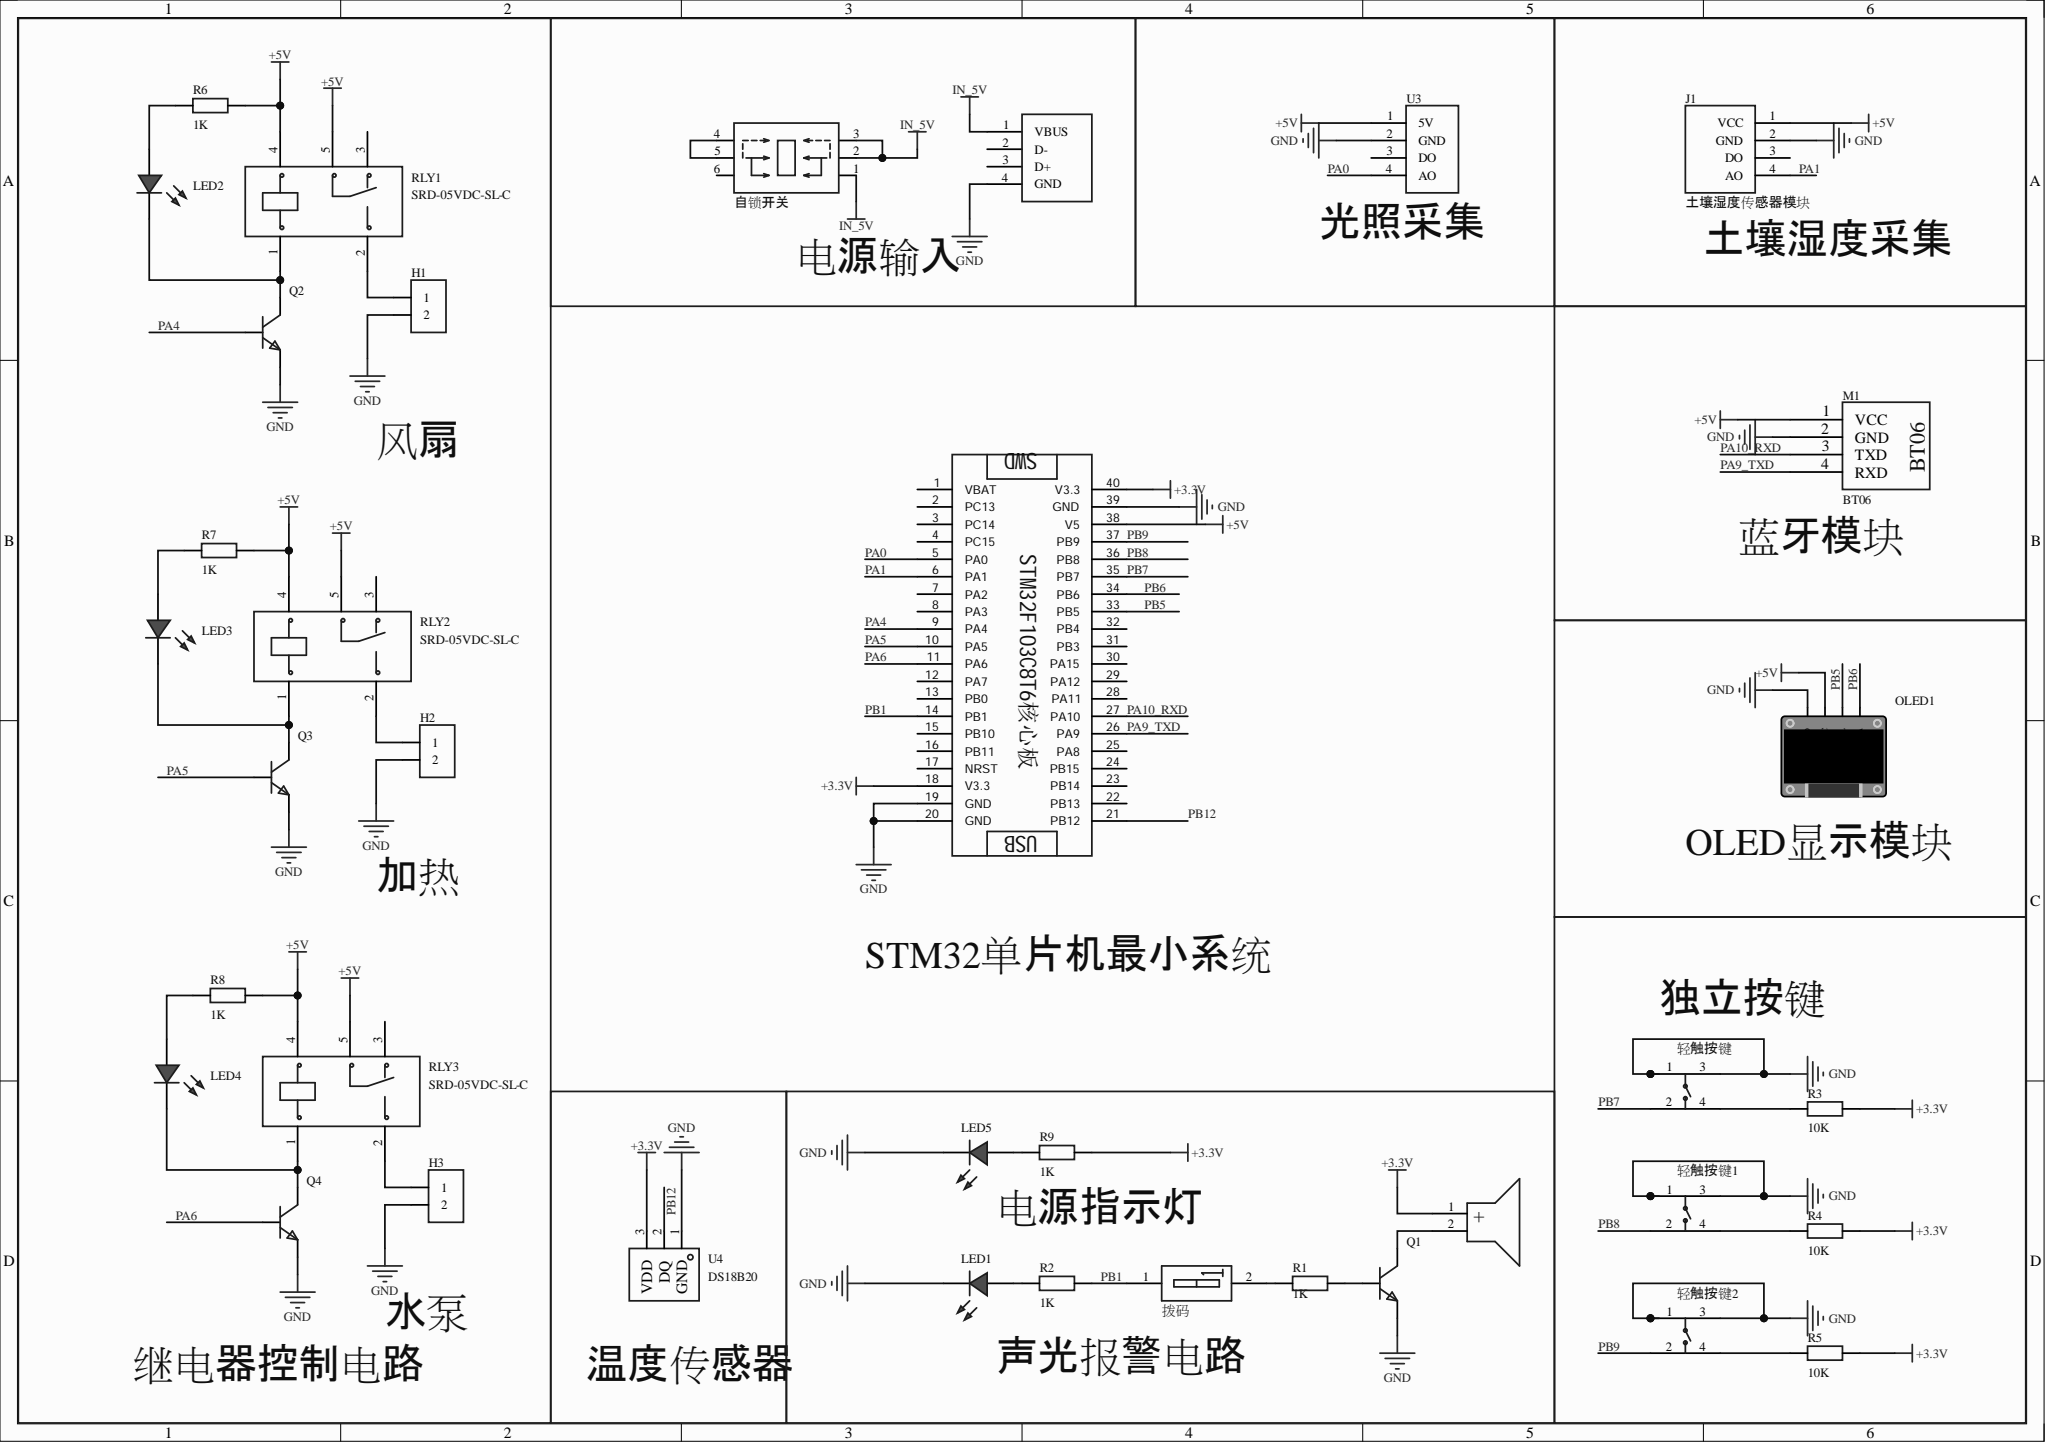Circuit board | Altium Designer | 37 parts | 36 nets
Bill of materials:
Comment,Description,Designator,Footprint,LibRef,Quantity
"3kHz","驱动方式:有源(内含驱动线路);构造类型:电磁式;频率:3kHz;声压(SPL):85dB;","BUZZER1","BUZ-TH_BD9.0-P5.00-D0.6-FD","HNB09A03","1"
"","","H1, H2, H3","HDR-TH_2P-P2.54-V-F","HDR-F_2.54_1x2P","3"
"土壤湿度传感器模块","","J1","Hearder-4","土壤湿度传感器模块","1"
"","","LED1, LED2, LED3, LED4, LED5","LED-TH_5mm","LED_TH-R_5mm","5"
"BT06","","M1","BT06","BT06","1"
"","","OLED1","0.96OLED_4P","0.96OLED模块_4P","1"
"S8050","晶体管类型:NPN;集电极电流(Ic):500mA;集射极击穿电压(Vceo):25V;耗散功率(Pd):300mW;直流电流增益(hFE):120@50mA,1.0V;","Q1, Q2, Q3, Q4","SOT-23-3_L2.9-W1.3-P1.90-LS2.3-BR","S8050_C20069125","4"
"1K","","R1, R2, R6, R7, R8, R9","R0805","Res_0805","6"
"10K","","R3, R4, R5","R0805","Res_0805","3"
"SRD-05VDC-SL-C","线圈电压:5V;触点形式:一组转换:1C(单刀双掷-转换);触点容量(电阻负载):-;最大切换电压:250V@AC;最大切换电流:15A;","RLY1, RLY2, RLY3","RELAY-TH_SRD-XXVDC-XL-C","SRD-05VDC-SL-C","3"
"自锁开关","8.5x8.5x14，6只端子、自锁、底座黑色、盖板灰色","SW1","SW-TH_6P-L8.5-W8.5-P2.50-LS5.5-BL-2","PS851-06L140E1-ZCY-G","1"
"拨码","类型:平拨,凸起式;电路结构:单刀单掷;开关位数:1位;工作寿命:-;颜色:红色;","SW2","SW-TH_DSWB01LHGET","DSWB01LHGET","1"
"","","U1","USB-type-C模块","TYPE-C模块","1"
"CW32F030C8最小系统板","","U2","STM32F103C8T6核心板","STM32F103C8T6最小系统","1"
"","","U3","光敏传感器模块","光敏传感器模块","1"
"DS18B20","","U4","3p_2.54","DS18B20","1"
"SH-6X6X6.5H-TP","电路结构:单刀单掷;按钮形状:圆形按钮;作用力:2.5N;安装方式:立贴;开关长度:6mm;开关宽度:6mm;开关高度:6.5mm;带支架:不带支架;触点电流:50mA;额定电压:12V;带灯:无;工作寿命:10万次;","轻触按键","SW-SMD_4P-L6.2-W6.2-P4.50-LS9.5-TL","SH-6X6X6.5H-TP","1"
"SH-6X6X6.5H-TP","电路结构:单刀单掷;按钮形状:圆形按钮;作用力:2.5N;安装方式:立贴;开关长度:6mm;开关宽度:6mm;开关高度:6.5mm;带支架:不带支架;触点电流:50mA;额定电压:12V;带灯:无;工作寿命:10万次;","轻触按键1, 轻触按键2","SW-SMD_4P-L6.0-W6.0-P4.50-LS8.8","SH-6X6X6.5H-TP","2"
Netlist (Protel format):
[
BUZZER1
BUZ-TH_BD9.0-P5.00-D0.6-FD
3kHz



]
[
H1
HDR-TH_2P-P2.54-V-F




]
[
H2
HDR-TH_2P-P2.54-V-F




]
[
H3
HDR-TH_2P-P2.54-V-F




]
[
J1
Hearder-4
土壤湿度传感器模块



]
[
LED1
LED-TH_5mm




]
[
LED2
LED-TH_5mm




]
[
LED3
LED-TH_5mm




]
[
LED4
LED-TH_5mm




]
[
LED5
LED-TH_5mm




]
[
M1
BT06
BT06



]
[
OLED1
0.96OLED_4P




]
[
Q1
SOT-23-3_L2.9-W1.3-P1.90-LS2.3-BR
S8050



]
[
Q2
SOT-23-3_L2.9-W1.3-P1.90-LS2.3-BR
S8050



]
[
Q3
SOT-23-3_L2.9-W1.3-P1.90-LS2.3-BR
S8050



]
[
Q4
SOT-23-3_L2.9-W1.3-P1.90-LS2.3-BR
S8050



]
[
R1
R0805
1K



]
[
R2
R0805
1K



]
[
R3
R0805
10K



]
[
R4
R0805
10K



]
[
R5
R0805
10K



]
[
R6
R0805
1K



]
[
R7
R0805
1K



]
[
R8
R0805
1K



]
[
R9
R0805
1K



]
[
RLY1
RELAY-TH_SRD-XXVDC-XL-C
SRD-05VDC-SL-C



]
[
RLY2
RELAY-TH_SRD-XXVDC-XL-C
SRD-05VDC-SL-C



]
[
RLY3
RELAY-TH_SRD-XXVDC-XL-C
SRD-05VDC-SL-C



]
[
SW1
SW-TH_6P-L8.5-W8.5-P2.50-LS5.5-BL-2
自锁开关



]
[
SW2
SW-TH_DSWB01LHGET
拨码



]
[
U1
USB-type-C模块




]
[
U2
STM32F103C8T6核心板
CW32F030C8最小系统板



]
[
U3
光敏传感器模块




]
[
U4
3p_2.54
DS18B20



]
[
轻触按键
SW-SMD_4P-L6.2-W6.2-P4.50-LS9.5-TL
SH-6X6X6.5H-TP



]
[
轻触按键1
SW-SMD_4P-L6.0-W6.0-P4.50-LS8.8
SH-6X6X6.5H-TP



]
[
轻触按键2
SW-SMD_4P-L6.0-W6.0-P4.50-LS8.8
SH-6X6X6.5H-TP



]
(
PB12
U2-21
U4-2
)
(
PB9
U2-37
轻触按键2-2
)
(
PB8
U2-36
轻触按键1-2
)
(
PB7
U2-35
轻触按键-2
)
(
PB6
OLED1-4
U2-34
)
(
PB5
OLED1-3
U2-33
)
(
PB1
R2-2
SW2-1
U2-14
)
(
PA10_RXD
M1-3
U2-27
)
(
PA9_TXD
M1-4
U2-26
)
(
PA6
Q4-1
U2-11
)
(
PA5
Q3-1
U2-10
)
(
PA4
Q2-1
U2-9
)
(
PA1
J1-4
U2-6
)
(
PA0
U2-5
U3-4
)
(
NetSW1_4
SW1-4
SW1-5
)
(
NetR5_1
R5-1
轻触按键2-4
)
(
NetR4_1
R4-1
轻触按键1-4
)
(
NetR3_1
R3-1
轻触按键-4
)
(
NetR1_1
R1-1
SW2-2
)
(
NetQ1_1
Q1-1
R1-2
)
(
NetLED5_1
LED5-1
R9-1
)
(
NetLED4_2
LED4-2
Q4-3
RLY3-1
)
(
NetLED4_1
LED4-1
R8-2
)
(
NetLED3_2
LED3-2
Q3-3
RLY2-1
)
(
NetLED3_1
LED3-1
R7-2
)
(
NetLED2_2
LED2-2
Q2-3
RLY1-1
)
(
NetLED2_1
LED2-1
R6-2
)
(
NetLED1_1
LED1-1
R2-1
)
(
NetH3_1
H3-1
RLY3-2
)
(
NetH2_1
H2-1
RLY2-2
)
(
NetH1_1
H1-1
RLY1-2
)
(
NetBUZZER1_2
BUZZER1-2
Q1-3
)
(
IN_5V
SW1-1
SW1-2
SW1-3
U1-1
)
(
GND
H1-2
H2-2
H3-2
J1-2
LED1-2
LED5-2
M1-2
OLED1-1
Q1-2
Q2-2
Q3-2
Q4-2
U1-4
U2-19
U2-20
U2-39
U3-2
U4-1
轻触按键-1
轻触按键-3
轻触按键1-1
轻触按键1-3
轻触按键2-1
轻触按键2-3
)
(
+5V
J1-1
M1-1
OLED1-2
R6-1
R7-1
R8-1
RLY1-4
RLY1-5
RLY2-4
RLY2-5
RLY3-4
RLY3-5
U2-38
U3-1
)
(
+3.3V
BUZZER1-1
R3-2
R4-2
R5-2
R9-2
U2-18
U2-40
U4-3
)